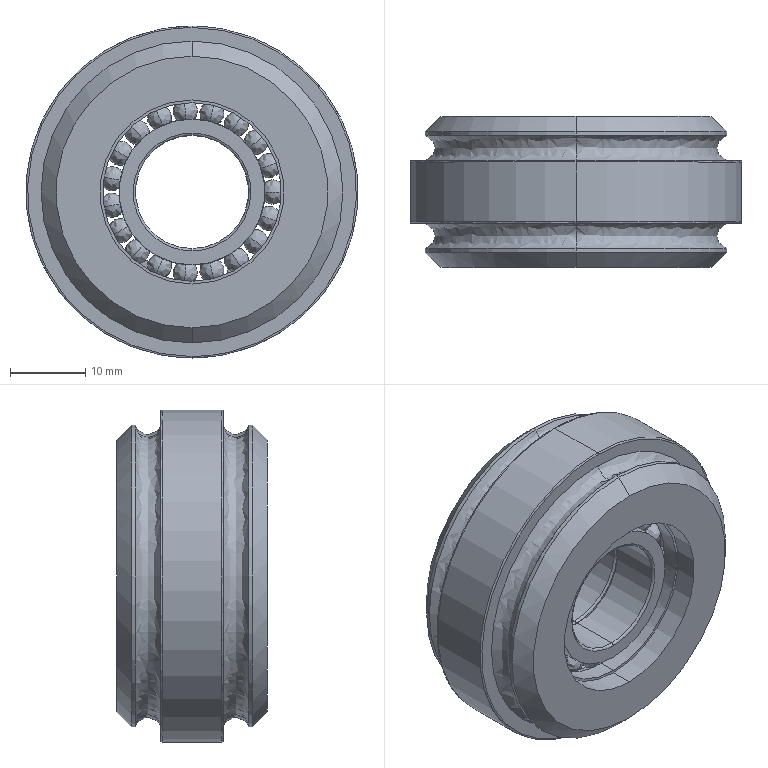Part | SolidWorks | 4 solids | 296 faces | box 44 x 20 x 44 mm | volume 18798 mm3 | spline 220 | cylinder 53 | plane 19 | cone 4 | commonest cylinder face diameters 19.333 x8 23.667 x8 28 x8 30.1 x5 2 x4 15 x4